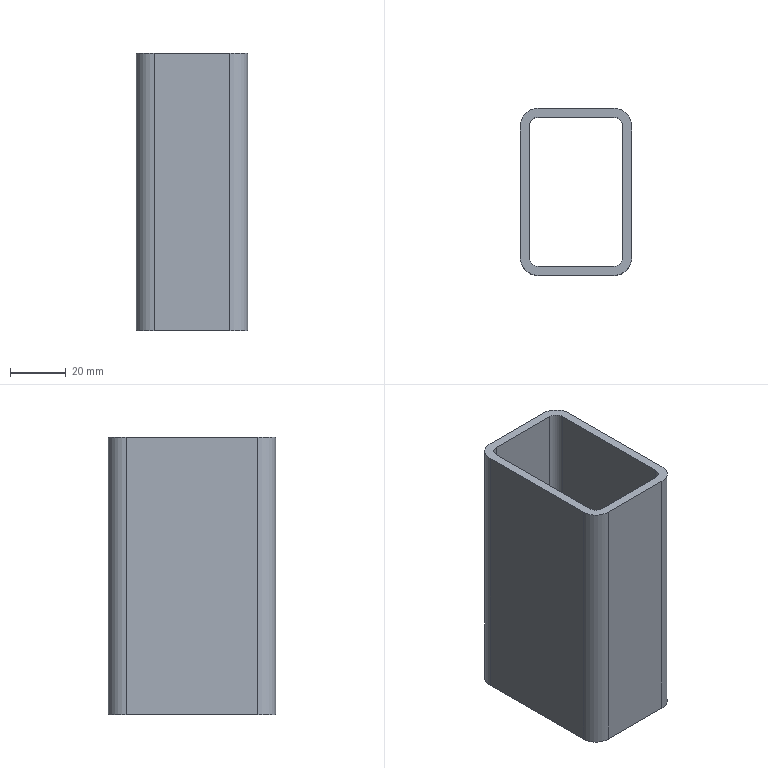Part | STEP file | Profile 4060100 | 1 solid | 18 faces | box 40 x 60 x 99.7 mm | volume 57095 mm3 | plane 10 | cylinder 8 | commonest cylinder face diameters 6.4 x4 12.8 x4
STEP:
#1=CARTESIAN_POINT('',(40.,6.4,-600.));
#2=VERTEX_POINT('',#1);
#3=CARTESIAN_POINT('',(40.,6.4,-500.3));
#4=VERTEX_POINT('',#3);
#5=CARTESIAN_POINT('',(40.,6.4,600.));
#6=DIRECTION('',(0.,0.,1.));
#7=VECTOR('',#6,1000.);
#8=LINE('',#5,#7);
#9=EDGE_CURVE('',#2,#4,#8,.T.);
#10=ORIENTED_EDGE('',*,*,#9,.F.);
#11=CARTESIAN_POINT('',(40.,53.6,-600.));
#12=VERTEX_POINT('',#11);
#13=CARTESIAN_POINT('',(40.,53.6,-600.));
#14=DIRECTION('',(0.,-1.,0.));
#15=VECTOR('',#14,1000.);
#16=LINE('',#13,#15);
#17=EDGE_CURVE('',#12,#2,#16,.T.);
#18=ORIENTED_EDGE('',*,*,#17,.F.);
#19=CARTESIAN_POINT('',(40.,53.6,-500.3));
#20=VERTEX_POINT('',#19);
#21=CARTESIAN_POINT('',(40.,53.6,600.));
#22=DIRECTION('',(0.,0.,-1.));
#23=VECTOR('',#22,1000.);
#24=LINE('',#21,#23);
#25=EDGE_CURVE('',#20,#12,#24,.T.);
#26=ORIENTED_EDGE('',*,*,#25,.F.);
#27=CARTESIAN_POINT('',(40.,53.6,-500.3));
#28=DIRECTION('',(0.,1.,0.));
#29=VECTOR('',#28,1000.);
#30=LINE('',#27,#29);
#31=EDGE_CURVE('',#4,#20,#30,.T.);
#32=ORIENTED_EDGE('',*,*,#31,.F.);
#33=EDGE_LOOP('',(#10,#18,#26,#32));
#34=FACE_OUTER_BOUND('',#33,.T.);
#35=CARTESIAN_POINT('',(40.,53.6,600.));
#36=DIRECTION('',(-1.,0.,0.));
#37=DIRECTION('',(0.,0.,1.));
#38=AXIS2_PLACEMENT_3D('',#35,#36,#37);
#39=PLANE('',#38);
#40=ADVANCED_FACE('',(#34),#39,.F.);
#41=CARTESIAN_POINT('',(0.,6.4,-500.3));
#42=VERTEX_POINT('',#41);
#43=CARTESIAN_POINT('',(6.4,0.,-500.3));
#44=VERTEX_POINT('',#43);
#45=CARTESIAN_POINT('',(6.4,6.4,-500.3));
#46=DIRECTION('',(0.,0.,1.));
#47=DIRECTION('',(-1.,0.,0.));
#48=AXIS2_PLACEMENT_3D('',#45,#46,#47);
#49=CIRCLE('',#48,6.4);
#50=EDGE_CURVE('',#42,#44,#49,.T.);
#51=ORIENTED_EDGE('',*,*,#50,.T.);
#52=CARTESIAN_POINT('',(33.6,0.,-500.3));
#53=VERTEX_POINT('',#52);
#54=CARTESIAN_POINT('',(33.6,0.,-500.3));
#55=DIRECTION('',(1.,0.,0.));
#56=VECTOR('',#55,1000.);
#57=LINE('',#54,#56);
#58=EDGE_CURVE('',#44,#53,#57,.T.);
#59=ORIENTED_EDGE('',*,*,#58,.T.);
#60=CARTESIAN_POINT('',(33.6,6.4,-500.3));
#61=DIRECTION('',(0.,0.,1.));
#62=DIRECTION('',(-1.,0.,0.));
#63=AXIS2_PLACEMENT_3D('',#60,#61,#62);
#64=CIRCLE('',#63,6.4);
#65=EDGE_CURVE('',#53,#4,#64,.T.);
#66=ORIENTED_EDGE('',*,*,#65,.T.);
#67=ORIENTED_EDGE('',*,*,#31,.T.);
#68=CARTESIAN_POINT('',(33.6,60.,-500.3));
#69=VERTEX_POINT('',#68);
#70=CARTESIAN_POINT('',(33.6,53.6,-500.3));
#71=DIRECTION('',(0.,0.,1.));
#72=DIRECTION('',(-1.,0.,0.));
#73=AXIS2_PLACEMENT_3D('',#70,#71,#72);
#74=CIRCLE('',#73,6.4);
#75=EDGE_CURVE('',#20,#69,#74,.T.);
#76=ORIENTED_EDGE('',*,*,#75,.T.);
#77=CARTESIAN_POINT('',(6.4,60.,-500.3));
#78=VERTEX_POINT('',#77);
#79=CARTESIAN_POINT('',(33.6,60.,-500.3));
#80=DIRECTION('',(-1.,0.,0.));
#81=VECTOR('',#80,1000.);
#82=LINE('',#79,#81);
#83=EDGE_CURVE('',#69,#78,#82,.T.);
#84=ORIENTED_EDGE('',*,*,#83,.T.);
#85=CARTESIAN_POINT('',(0.,53.6,-500.3));
#86=VERTEX_POINT('',#85);
#87=CARTESIAN_POINT('',(6.4,53.6,-500.3));
#88=DIRECTION('',(0.,0.,1.));
#89=DIRECTION('',(-1.,0.,0.));
#90=AXIS2_PLACEMENT_3D('',#87,#88,#89);
#91=CIRCLE('',#90,6.4);
#92=EDGE_CURVE('',#78,#86,#91,.T.);
#93=ORIENTED_EDGE('',*,*,#92,.T.);
#94=CARTESIAN_POINT('',(0.,6.4,-500.3));
#95=DIRECTION('',(0.,-1.,0.));
#96=VECTOR('',#95,1000.);
#97=LINE('',#94,#96);
#98=EDGE_CURVE('',#86,#42,#97,.T.);
#99=ORIENTED_EDGE('',*,*,#98,.T.);
#100=EDGE_LOOP('',(#51,#59,#66,#67,#76,#84,#93,#99));
#101=FACE_OUTER_BOUND('',#100,.T.);
#102=CARTESIAN_POINT('',(3.2,53.6,-500.3));
#103=VERTEX_POINT('',#102);
#104=CARTESIAN_POINT('',(6.4,56.8,-500.3));
#105=VERTEX_POINT('',#104);
#106=CARTESIAN_POINT('',(6.4,53.6,-500.3));
#107=DIRECTION('',(0.,0.,-1.));
#108=DIRECTION('',(-1.,0.,0.));
#109=AXIS2_PLACEMENT_3D('',#106,#107,#108);
#110=CIRCLE('',#109,3.2);
#111=EDGE_CURVE('',#103,#105,#110,.T.);
#112=ORIENTED_EDGE('',*,*,#111,.T.);
#113=CARTESIAN_POINT('',(33.6,56.8,-500.3));
#114=VERTEX_POINT('',#113);
#115=CARTESIAN_POINT('',(33.6,56.8,-500.3));
#116=DIRECTION('',(1.,0.,0.));
#117=VECTOR('',#116,1000.);
#118=LINE('',#115,#117);
#119=EDGE_CURVE('',#105,#114,#118,.T.);
#120=ORIENTED_EDGE('',*,*,#119,.T.);
#121=CARTESIAN_POINT('',(36.8,53.6,-500.3));
#122=VERTEX_POINT('',#121);
#123=CARTESIAN_POINT('',(33.6,53.6,-500.3));
#124=DIRECTION('',(0.,0.,-1.));
#125=DIRECTION('',(-1.,0.,0.));
#126=AXIS2_PLACEMENT_3D('',#123,#124,#125);
#127=CIRCLE('',#126,3.2);
#128=EDGE_CURVE('',#114,#122,#127,.T.);
#129=ORIENTED_EDGE('',*,*,#128,.T.);
#130=CARTESIAN_POINT('',(36.8,6.4,-500.3));
#131=VERTEX_POINT('',#130);
#132=CARTESIAN_POINT('',(36.8,6.4,-500.3));
#133=DIRECTION('',(0.,-1.,0.));
#134=VECTOR('',#133,1000.);
#135=LINE('',#132,#134);
#136=EDGE_CURVE('',#122,#131,#135,.T.);
#137=ORIENTED_EDGE('',*,*,#136,.T.);
#138=CARTESIAN_POINT('',(33.6,3.2,-500.3));
#139=VERTEX_POINT('',#138);
#140=CARTESIAN_POINT('',(33.6,6.4,-500.3));
#141=DIRECTION('',(0.,0.,-1.));
#142=DIRECTION('',(-1.,0.,0.));
#143=AXIS2_PLACEMENT_3D('',#140,#141,#142);
#144=CIRCLE('',#143,3.2);
#145=EDGE_CURVE('',#131,#139,#144,.T.);
#146=ORIENTED_EDGE('',*,*,#145,.T.);
#147=CARTESIAN_POINT('',(6.4,3.2,-500.3));
#148=VERTEX_POINT('',#147);
#149=CARTESIAN_POINT('',(33.6,3.2,-500.3));
#150=DIRECTION('',(-1.,0.,0.));
#151=VECTOR('',#150,1000.);
#152=LINE('',#149,#151);
#153=EDGE_CURVE('',#139,#148,#152,.T.);
#154=ORIENTED_EDGE('',*,*,#153,.T.);
#155=CARTESIAN_POINT('',(3.2,6.4,-500.3));
#156=VERTEX_POINT('',#155);
#157=CARTESIAN_POINT('',(6.4,6.4,-500.3));
#158=DIRECTION('',(0.,0.,-1.));
#159=DIRECTION('',(-1.,0.,0.));
#160=AXIS2_PLACEMENT_3D('',#157,#158,#159);
#161=CIRCLE('',#160,3.2);
#162=EDGE_CURVE('',#148,#156,#161,.T.);
#163=ORIENTED_EDGE('',*,*,#162,.T.);
#164=CARTESIAN_POINT('',(3.2,6.4,-500.3));
#165=DIRECTION('',(0.,1.,0.));
#166=VECTOR('',#165,1000.);
#167=LINE('',#164,#166);
#168=EDGE_CURVE('',#156,#103,#167,.T.);
#169=ORIENTED_EDGE('',*,*,#168,.T.);
#170=EDGE_LOOP('',(#112,#120,#129,#137,#146,#154,#163,#169));
#171=FACE_BOUND('',#170,.T.);
#172=CARTESIAN_POINT('',(33.6,6.4,-500.3));
#173=DIRECTION('',(0.,0.,1.));
#174=DIRECTION('',(1.,0.,0.));
#175=AXIS2_PLACEMENT_3D('',#172,#173,#174);
#176=PLANE('',#175);
#177=ADVANCED_FACE('',(#101,#171),#176,.T.);
#178=CARTESIAN_POINT('',(33.6,0.,-600.));
#179=VERTEX_POINT('',#178);
#180=CARTESIAN_POINT('',(33.6,0.,600.));
#181=DIRECTION('',(0.,0.,-1.));
#182=VECTOR('',#181,1000.);
#183=LINE('',#180,#182);
#184=EDGE_CURVE('',#53,#179,#183,.T.);
#185=ORIENTED_EDGE('',*,*,#184,.T.);
#186=CARTESIAN_POINT('',(33.6,6.4,-600.));
#187=DIRECTION('',(0.,0.,1.));
#188=DIRECTION('',(-1.,0.,0.));
#189=AXIS2_PLACEMENT_3D('',#186,#187,#188);
#190=CIRCLE('',#189,6.4);
#191=EDGE_CURVE('',#179,#2,#190,.T.);
#192=ORIENTED_EDGE('',*,*,#191,.T.);
#193=ORIENTED_EDGE('',*,*,#9,.T.);
#194=ORIENTED_EDGE('',*,*,#65,.F.);
#195=EDGE_LOOP('',(#185,#192,#193,#194));
#196=FACE_OUTER_BOUND('',#195,.T.);
#197=CARTESIAN_POINT('',(33.6,6.4,600.));
#198=DIRECTION('',(0.,0.,-1.));
#199=DIRECTION('',(-1.,0.,0.));
#200=AXIS2_PLACEMENT_3D('',#197,#198,#199);
#201=CYLINDRICAL_SURFACE('',#200,6.4);
#202=ADVANCED_FACE('',(#196),#201,.T.);
#203=ORIENTED_EDGE('',*,*,#191,.F.);
#204=CARTESIAN_POINT('',(6.4,0.,-600.));
#205=VERTEX_POINT('',#204);
#206=CARTESIAN_POINT('',(33.6,0.,-600.));
#207=DIRECTION('',(1.,0.,0.));
#208=VECTOR('',#207,1000.);
#209=LINE('',#206,#208);
#210=EDGE_CURVE('',#205,#179,#209,.T.);
#211=ORIENTED_EDGE('',*,*,#210,.F.);
#212=CARTESIAN_POINT('',(0.,6.4,-600.));
#213=VERTEX_POINT('',#212);
#214=CARTESIAN_POINT('',(6.4,6.4,-600.));
#215=DIRECTION('',(0.,0.,1.));
#216=DIRECTION('',(-1.,0.,0.));
#217=AXIS2_PLACEMENT_3D('',#214,#215,#216);
#218=CIRCLE('',#217,6.4);
#219=EDGE_CURVE('',#213,#205,#218,.T.);
#220=ORIENTED_EDGE('',*,*,#219,.F.);
#221=CARTESIAN_POINT('',(0.,53.6,-600.));
#222=VERTEX_POINT('',#221);
#223=CARTESIAN_POINT('',(0.,53.6,-600.));
#224=DIRECTION('',(0.,-1.,0.));
#225=VECTOR('',#224,1000.);
#226=LINE('',#223,#225);
#227=EDGE_CURVE('',#222,#213,#226,.T.);
#228=ORIENTED_EDGE('',*,*,#227,.F.);
#229=CARTESIAN_POINT('',(6.4,60.,-600.));
#230=VERTEX_POINT('',#229);
#231=CARTESIAN_POINT('',(6.4,53.6,-600.));
#232=DIRECTION('',(0.,0.,1.));
#233=DIRECTION('',(-1.,0.,0.));
#234=AXIS2_PLACEMENT_3D('',#231,#232,#233);
#235=CIRCLE('',#234,6.4);
#236=EDGE_CURVE('',#230,#222,#235,.T.);
#237=ORIENTED_EDGE('',*,*,#236,.F.);
#238=CARTESIAN_POINT('',(33.6,60.,-600.));
#239=VERTEX_POINT('',#238);
#240=CARTESIAN_POINT('',(33.6,60.,-600.));
#241=DIRECTION('',(-1.,0.,0.));
#242=VECTOR('',#241,1000.);
#243=LINE('',#240,#242);
#244=EDGE_CURVE('',#239,#230,#243,.T.);
#245=ORIENTED_EDGE('',*,*,#244,.F.);
#246=CARTESIAN_POINT('',(33.6,53.6,-600.));
#247=DIRECTION('',(0.,0.,1.));
#248=DIRECTION('',(-1.,0.,0.));
#249=AXIS2_PLACEMENT_3D('',#246,#247,#248);
#250=CIRCLE('',#249,6.4);
#251=EDGE_CURVE('',#12,#239,#250,.T.);
#252=ORIENTED_EDGE('',*,*,#251,.F.);
#253=ORIENTED_EDGE('',*,*,#17,.T.);
#254=EDGE_LOOP('',(#203,#211,#220,#228,#237,#245,#252,#253));
#255=FACE_OUTER_BOUND('',#254,.T.);
#256=CARTESIAN_POINT('',(6.4,3.2,-600.));
#257=VERTEX_POINT('',#256);
#258=CARTESIAN_POINT('',(3.2,6.4,-600.));
#259=VERTEX_POINT('',#258);
#260=CARTESIAN_POINT('',(6.4,6.4,-600.));
#261=DIRECTION('',(0.,0.,-1.));
#262=DIRECTION('',(-1.,0.,0.));
#263=AXIS2_PLACEMENT_3D('',#260,#261,#262);
#264=CIRCLE('',#263,3.2);
#265=EDGE_CURVE('',#257,#259,#264,.T.);
#266=ORIENTED_EDGE('',*,*,#265,.F.);
#267=CARTESIAN_POINT('',(33.6,3.2,-600.));
#268=VERTEX_POINT('',#267);
#269=CARTESIAN_POINT('',(33.6,3.2,-600.));
#270=DIRECTION('',(-1.,0.,0.));
#271=VECTOR('',#270,1000.);
#272=LINE('',#269,#271);
#273=EDGE_CURVE('',#268,#257,#272,.T.);
#274=ORIENTED_EDGE('',*,*,#273,.F.);
#275=CARTESIAN_POINT('',(36.8,6.4,-600.));
#276=VERTEX_POINT('',#275);
#277=CARTESIAN_POINT('',(33.6,6.4,-600.));
#278=DIRECTION('',(0.,0.,-1.));
#279=DIRECTION('',(-1.,0.,0.));
#280=AXIS2_PLACEMENT_3D('',#277,#278,#279);
#281=CIRCLE('',#280,3.2);
#282=EDGE_CURVE('',#276,#268,#281,.T.);
#283=ORIENTED_EDGE('',*,*,#282,.F.);
#284=CARTESIAN_POINT('',(36.8,53.6,-600.));
#285=VERTEX_POINT('',#284);
#286=CARTESIAN_POINT('',(36.8,53.6,-600.));
#287=DIRECTION('',(0.,-1.,0.));
#288=VECTOR('',#287,1000.);
#289=LINE('',#286,#288);
#290=EDGE_CURVE('',#285,#276,#289,.T.);
#291=ORIENTED_EDGE('',*,*,#290,.F.);
#292=CARTESIAN_POINT('',(33.6,56.8,-600.));
#293=VERTEX_POINT('',#292);
#294=CARTESIAN_POINT('',(33.6,53.6,-600.));
#295=DIRECTION('',(0.,0.,-1.));
#296=DIRECTION('',(-1.,0.,0.));
#297=AXIS2_PLACEMENT_3D('',#294,#295,#296);
#298=CIRCLE('',#297,3.2);
#299=EDGE_CURVE('',#293,#285,#298,.T.);
#300=ORIENTED_EDGE('',*,*,#299,.F.);
#301=CARTESIAN_POINT('',(6.4,56.8,-600.));
#302=VERTEX_POINT('',#301);
#303=CARTESIAN_POINT('',(33.6,56.8,-600.));
#304=DIRECTION('',(1.,0.,0.));
#305=VECTOR('',#304,1000.);
#306=LINE('',#303,#305);
#307=EDGE_CURVE('',#302,#293,#306,.T.);
#308=ORIENTED_EDGE('',*,*,#307,.F.);
#309=CARTESIAN_POINT('',(3.2,53.6,-600.));
#310=VERTEX_POINT('',#309);
#311=CARTESIAN_POINT('',(6.4,53.6,-600.));
#312=DIRECTION('',(0.,0.,-1.));
#313=DIRECTION('',(-1.,0.,0.));
#314=AXIS2_PLACEMENT_3D('',#311,#312,#313);
#315=CIRCLE('',#314,3.2);
#316=EDGE_CURVE('',#310,#302,#315,.T.);
#317=ORIENTED_EDGE('',*,*,#316,.F.);
#318=CARTESIAN_POINT('',(3.2,53.6,-600.));
#319=DIRECTION('',(0.,1.,0.));
#320=VECTOR('',#319,1000.);
#321=LINE('',#318,#320);
#322=EDGE_CURVE('',#259,#310,#321,.T.);
#323=ORIENTED_EDGE('',*,*,#322,.F.);
#324=EDGE_LOOP('',(#266,#274,#283,#291,#300,#308,#317,#323));
#325=FACE_BOUND('',#324,.T.);
#326=CARTESIAN_POINT('',(33.6,53.6,-600.));
#327=DIRECTION('',(0.,0.,1.));
#328=DIRECTION('',(1.,0.,0.));
#329=AXIS2_PLACEMENT_3D('',#326,#327,#328);
#330=PLANE('',#329);
#331=ADVANCED_FACE('',(#255,#325),#330,.F.);
#332=ORIENTED_EDGE('',*,*,#25,.T.);
#333=ORIENTED_EDGE('',*,*,#251,.T.);
#334=CARTESIAN_POINT('',(33.6,60.,600.));
#335=DIRECTION('',(0.,0.,1.));
#336=VECTOR('',#335,1000.);
#337=LINE('',#334,#336);
#338=EDGE_CURVE('',#239,#69,#337,.T.);
#339=ORIENTED_EDGE('',*,*,#338,.T.);
#340=ORIENTED_EDGE('',*,*,#75,.F.);
#341=EDGE_LOOP('',(#332,#333,#339,#340));
#342=FACE_OUTER_BOUND('',#341,.T.);
#343=CARTESIAN_POINT('',(33.6,53.6,600.));
#344=DIRECTION('',(0.,0.,-1.));
#345=DIRECTION('',(-1.,0.,0.));
#346=AXIS2_PLACEMENT_3D('',#343,#344,#345);
#347=CYLINDRICAL_SURFACE('',#346,6.4);
#348=ADVANCED_FACE('',(#342),#347,.T.);
#349=CARTESIAN_POINT('',(6.4,0.,600.));
#350=DIRECTION('',(0.,0.,1.));
#351=VECTOR('',#350,1000.);
#352=LINE('',#349,#351);
#353=EDGE_CURVE('',#205,#44,#352,.T.);
#354=ORIENTED_EDGE('',*,*,#353,.F.);
#355=ORIENTED_EDGE('',*,*,#210,.T.);
#356=ORIENTED_EDGE('',*,*,#184,.F.);
#357=ORIENTED_EDGE('',*,*,#58,.F.);
#358=EDGE_LOOP('',(#354,#355,#356,#357));
#359=FACE_OUTER_BOUND('',#358,.T.);
#360=CARTESIAN_POINT('',(6.4,0.,600.));
#361=DIRECTION('',(0.,1.,0.));
#362=DIRECTION('',(-1.,0.,0.));
#363=AXIS2_PLACEMENT_3D('',#360,#361,#362);
#364=PLANE('',#363);
#365=ADVANCED_FACE('',(#359),#364,.F.);
#366=CARTESIAN_POINT('',(0.,6.4,600.));
#367=DIRECTION('',(0.,0.,-1.));
#368=VECTOR('',#367,1000.);
#369=LINE('',#366,#368);
#370=EDGE_CURVE('',#42,#213,#369,.T.);
#371=ORIENTED_EDGE('',*,*,#370,.T.);
#372=ORIENTED_EDGE('',*,*,#219,.T.);
#373=ORIENTED_EDGE('',*,*,#353,.T.);
#374=ORIENTED_EDGE('',*,*,#50,.F.);
#375=EDGE_LOOP('',(#371,#372,#373,#374));
#376=FACE_OUTER_BOUND('',#375,.T.);
#377=CARTESIAN_POINT('',(6.4,6.4,600.));
#378=DIRECTION('',(0.,0.,-1.));
#379=DIRECTION('',(-1.,0.,0.));
#380=AXIS2_PLACEMENT_3D('',#377,#378,#379);
#381=CYLINDRICAL_SURFACE('',#380,6.4);
#382=ADVANCED_FACE('',(#376),#381,.T.);
#383=CARTESIAN_POINT('',(0.,53.6,600.));
#384=DIRECTION('',(0.,0.,1.));
#385=VECTOR('',#384,1000.);
#386=LINE('',#383,#385);
#387=EDGE_CURVE('',#222,#86,#386,.T.);
#388=ORIENTED_EDGE('',*,*,#387,.F.);
#389=ORIENTED_EDGE('',*,*,#227,.T.);
#390=ORIENTED_EDGE('',*,*,#370,.F.);
#391=ORIENTED_EDGE('',*,*,#98,.F.);
#392=EDGE_LOOP('',(#388,#389,#390,#391));
#393=FACE_OUTER_BOUND('',#392,.T.);
#394=CARTESIAN_POINT('',(0.,6.4,600.));
#395=DIRECTION('',(1.,0.,0.));
#396=DIRECTION('',(0.,1.,0.));
#397=AXIS2_PLACEMENT_3D('',#394,#395,#396);
#398=PLANE('',#397);
#399=ADVANCED_FACE('',(#393),#398,.F.);
#400=CARTESIAN_POINT('',(6.4,60.,600.));
#401=DIRECTION('',(0.,0.,-1.));
#402=VECTOR('',#401,1000.);
#403=LINE('',#400,#402);
#404=EDGE_CURVE('',#78,#230,#403,.T.);
#405=ORIENTED_EDGE('',*,*,#404,.T.);
#406=ORIENTED_EDGE('',*,*,#236,.T.);
#407=ORIENTED_EDGE('',*,*,#387,.T.);
#408=ORIENTED_EDGE('',*,*,#92,.F.);
#409=EDGE_LOOP('',(#405,#406,#407,#408));
#410=FACE_OUTER_BOUND('',#409,.T.);
#411=CARTESIAN_POINT('',(6.4,53.6,600.));
#412=DIRECTION('',(0.,0.,-1.));
#413=DIRECTION('',(-1.,0.,0.));
#414=AXIS2_PLACEMENT_3D('',#411,#412,#413);
#415=CYLINDRICAL_SURFACE('',#414,6.4);
#416=ADVANCED_FACE('',(#410),#415,.T.);
#417=ORIENTED_EDGE('',*,*,#338,.F.);
#418=ORIENTED_EDGE('',*,*,#244,.T.);
#419=ORIENTED_EDGE('',*,*,#404,.F.);
#420=ORIENTED_EDGE('',*,*,#83,.F.);
#421=EDGE_LOOP('',(#417,#418,#419,#420));
#422=FACE_OUTER_BOUND('',#421,.T.);
#423=CARTESIAN_POINT('',(33.6,60.,600.));
#424=DIRECTION('',(0.,-1.,0.));
#425=DIRECTION('',(0.,0.,-1.));
#426=AXIS2_PLACEMENT_3D('',#423,#424,#425);
#427=PLANE('',#426);
#428=ADVANCED_FACE('',(#422),#427,.F.);
#429=CARTESIAN_POINT('',(6.4,56.8,600.));
#430=DIRECTION('',(0.,0.,-1.));
#431=VECTOR('',#430,1000.);
#432=LINE('',#429,#431);
#433=EDGE_CURVE('',#105,#302,#432,.T.);
#434=ORIENTED_EDGE('',*,*,#433,.T.);
#435=ORIENTED_EDGE('',*,*,#307,.T.);
#436=CARTESIAN_POINT('',(33.6,56.8,600.));
#437=DIRECTION('',(0.,0.,1.));
#438=VECTOR('',#437,1000.);
#439=LINE('',#436,#438);
#440=EDGE_CURVE('',#293,#114,#439,.T.);
#441=ORIENTED_EDGE('',*,*,#440,.T.);
#442=ORIENTED_EDGE('',*,*,#119,.F.);
#443=EDGE_LOOP('',(#434,#435,#441,#442));
#444=FACE_OUTER_BOUND('',#443,.T.);
#445=CARTESIAN_POINT('',(33.6,56.8,600.));
#446=DIRECTION('',(0.,-1.,0.));
#447=DIRECTION('',(0.,0.,-1.));
#448=AXIS2_PLACEMENT_3D('',#445,#446,#447);
#449=PLANE('',#448);
#450=ADVANCED_FACE('',(#444),#449,.T.);
#451=CARTESIAN_POINT('',(3.2,53.6,600.));
#452=DIRECTION('',(0.,0.,1.));
#453=VECTOR('',#452,1000.);
#454=LINE('',#451,#453);
#455=EDGE_CURVE('',#310,#103,#454,.T.);
#456=ORIENTED_EDGE('',*,*,#455,.F.);
#457=ORIENTED_EDGE('',*,*,#316,.T.);
#458=ORIENTED_EDGE('',*,*,#433,.F.);
#459=ORIENTED_EDGE('',*,*,#111,.F.);
#460=EDGE_LOOP('',(#456,#457,#458,#459));
#461=FACE_OUTER_BOUND('',#460,.T.);
#462=CARTESIAN_POINT('',(6.4,53.6,600.));
#463=DIRECTION('',(0.,0.,-1.));
#464=DIRECTION('',(-1.,0.,0.));
#465=AXIS2_PLACEMENT_3D('',#462,#463,#464);
#466=CYLINDRICAL_SURFACE('',#465,3.2);
#467=ADVANCED_FACE('',(#461),#466,.F.);
#468=CARTESIAN_POINT('',(3.2,6.4,600.));
#469=DIRECTION('',(0.,0.,-1.));
#470=VECTOR('',#469,1000.);
#471=LINE('',#468,#470);
#472=EDGE_CURVE('',#156,#259,#471,.T.);
#473=ORIENTED_EDGE('',*,*,#472,.T.);
#474=ORIENTED_EDGE('',*,*,#322,.T.);
#475=ORIENTED_EDGE('',*,*,#455,.T.);
#476=ORIENTED_EDGE('',*,*,#168,.F.);
#477=EDGE_LOOP('',(#473,#474,#475,#476));
#478=FACE_OUTER_BOUND('',#477,.T.);
#479=CARTESIAN_POINT('',(3.2,6.4,600.));
#480=DIRECTION('',(1.,0.,0.));
#481=DIRECTION('',(0.,1.,0.));
#482=AXIS2_PLACEMENT_3D('',#479,#480,#481);
#483=PLANE('',#482);
#484=ADVANCED_FACE('',(#478),#483,.T.);
#485=CARTESIAN_POINT('',(6.4,3.2,600.));
#486=DIRECTION('',(0.,0.,1.));
#487=VECTOR('',#486,1000.);
#488=LINE('',#485,#487);
#489=EDGE_CURVE('',#257,#148,#488,.T.);
#490=ORIENTED_EDGE('',*,*,#489,.F.);
#491=ORIENTED_EDGE('',*,*,#265,.T.);
#492=ORIENTED_EDGE('',*,*,#472,.F.);
#493=ORIENTED_EDGE('',*,*,#162,.F.);
#494=EDGE_LOOP('',(#490,#491,#492,#493));
#495=FACE_OUTER_BOUND('',#494,.T.);
#496=CARTESIAN_POINT('',(6.4,6.4,600.));
#497=DIRECTION('',(0.,0.,-1.));
#498=DIRECTION('',(-1.,0.,0.));
#499=AXIS2_PLACEMENT_3D('',#496,#497,#498);
#500=CYLINDRICAL_SURFACE('',#499,3.2);
#501=ADVANCED_FACE('',(#495),#500,.F.);
#502=CARTESIAN_POINT('',(33.6,3.2,600.));
#503=DIRECTION('',(0.,0.,-1.));
#504=VECTOR('',#503,1000.);
#505=LINE('',#502,#504);
#506=EDGE_CURVE('',#139,#268,#505,.T.);
#507=ORIENTED_EDGE('',*,*,#506,.T.);
#508=ORIENTED_EDGE('',*,*,#273,.T.);
#509=ORIENTED_EDGE('',*,*,#489,.T.);
#510=ORIENTED_EDGE('',*,*,#153,.F.);
#511=EDGE_LOOP('',(#507,#508,#509,#510));
#512=FACE_OUTER_BOUND('',#511,.T.);
#513=CARTESIAN_POINT('',(6.4,3.2,600.));
#514=DIRECTION('',(0.,1.,0.));
#515=DIRECTION('',(-1.,0.,0.));
#516=AXIS2_PLACEMENT_3D('',#513,#514,#515);
#517=PLANE('',#516);
#518=ADVANCED_FACE('',(#512),#517,.T.);
#519=CARTESIAN_POINT('',(36.8,6.4,600.));
#520=DIRECTION('',(0.,0.,1.));
#521=VECTOR('',#520,1000.);
#522=LINE('',#519,#521);
#523=EDGE_CURVE('',#276,#131,#522,.T.);
#524=ORIENTED_EDGE('',*,*,#523,.F.);
#525=ORIENTED_EDGE('',*,*,#282,.T.);
#526=ORIENTED_EDGE('',*,*,#506,.F.);
#527=ORIENTED_EDGE('',*,*,#145,.F.);
#528=EDGE_LOOP('',(#524,#525,#526,#527));
#529=FACE_OUTER_BOUND('',#528,.T.);
#530=CARTESIAN_POINT('',(33.6,6.4,600.));
#531=DIRECTION('',(0.,0.,-1.));
#532=DIRECTION('',(-1.,0.,0.));
#533=AXIS2_PLACEMENT_3D('',#530,#531,#532);
#534=CYLINDRICAL_SURFACE('',#533,3.2);
#535=ADVANCED_FACE('',(#529),#534,.F.);
#536=CARTESIAN_POINT('',(36.8,53.6,600.));
#537=DIRECTION('',(0.,0.,-1.));
#538=VECTOR('',#537,1000.);
#539=LINE('',#536,#538);
#540=EDGE_CURVE('',#122,#285,#539,.T.);
#541=ORIENTED_EDGE('',*,*,#540,.T.);
#542=ORIENTED_EDGE('',*,*,#290,.T.);
#543=ORIENTED_EDGE('',*,*,#523,.T.);
#544=ORIENTED_EDGE('',*,*,#136,.F.);
#545=EDGE_LOOP('',(#541,#542,#543,#544));
#546=FACE_OUTER_BOUND('',#545,.T.);
#547=CARTESIAN_POINT('',(36.8,53.6,600.));
#548=DIRECTION('',(-1.,0.,0.));
#549=DIRECTION('',(0.,0.,1.));
#550=AXIS2_PLACEMENT_3D('',#547,#548,#549);
#551=PLANE('',#550);
#552=ADVANCED_FACE('',(#546),#551,.T.);
#553=ORIENTED_EDGE('',*,*,#440,.F.);
#554=ORIENTED_EDGE('',*,*,#299,.T.);
#555=ORIENTED_EDGE('',*,*,#540,.F.);
#556=ORIENTED_EDGE('',*,*,#128,.F.);
#557=EDGE_LOOP('',(#553,#554,#555,#556));
#558=FACE_OUTER_BOUND('',#557,.T.);
#559=CARTESIAN_POINT('',(33.6,53.6,600.));
#560=DIRECTION('',(0.,0.,-1.));
#561=DIRECTION('',(-1.,0.,0.));
#562=AXIS2_PLACEMENT_3D('',#559,#560,#561);
#563=CYLINDRICAL_SURFACE('',#562,3.2);
#564=ADVANCED_FACE('',(#558),#563,.F.);
#565=CLOSED_SHELL('',(#40,#177,#202,#331,#348,#365,#382,#399,#416,#428,#450,#467,#484,#501,#518,#535,#552,#564));
#566=MANIFOLD_SOLID_BREP('',#565);
#567=CARTESIAN_POINT('',(0.,0.,0.));
#568=DIRECTION('',(0.,0.,1.));
#569=DIRECTION('',(1.,0.,0.));
#570=AXIS2_PLACEMENT_3D('',#567,#568,#569);
#571=(LENGTH_UNIT()NAMED_UNIT(*)SI_UNIT(.MILLI.,.METRE.));
#572=UNCERTAINTY_MEASURE_WITH_UNIT(LENGTH_MEASURE(0.00001),#571,'','');
#573=(NAMED_UNIT(*)PLANE_ANGLE_UNIT()SI_UNIT($,.RADIAN.));
#574=(NAMED_UNIT(*)SI_UNIT($,.STERADIAN.)SOLID_ANGLE_UNIT());
#575=(GEOMETRIC_REPRESENTATION_CONTEXT(3)GLOBAL_UNCERTAINTY_ASSIGNED_CONTEXT((#572))GLOBAL_UNIT_ASSIGNED_CONTEXT((#571,#573,#574))REPRESENTATION_CONTEXT('',''));
#576=ADVANCED_BREP_SHAPE_REPRESENTATION('',(#566,#570),#575);